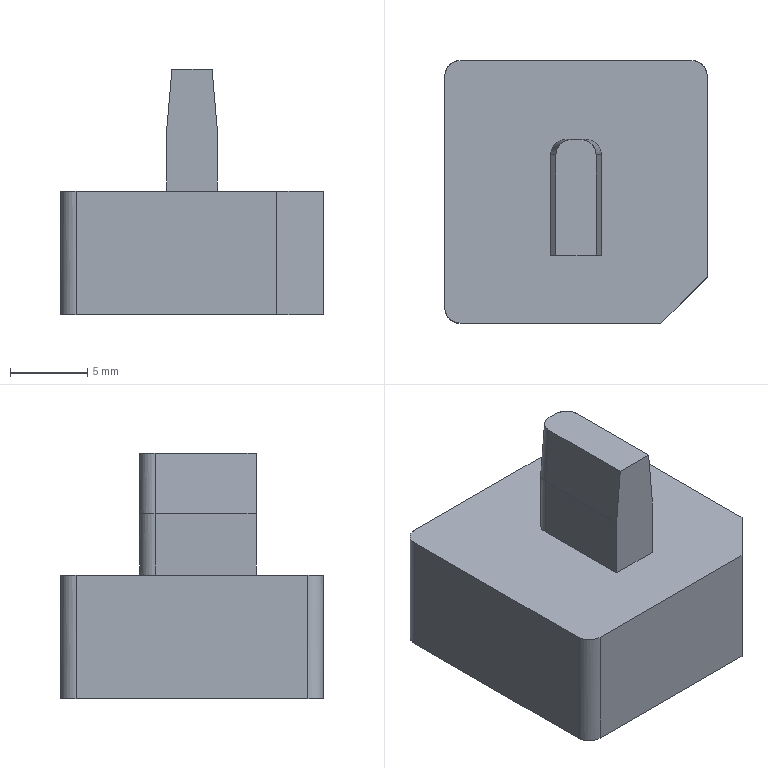NC program | PowerMill | posted with a generic post | part box 17 x 17 x 15.883 mm
Lines 1 to 1090 of 22972:
%
O0001
N104 ( POWERMILL CB  : 2026004.0)
N105 ( POST VER      : 2026.0.0.5161)
N106 ( OPTION FILE   : FANUC)
N107 ( OUTPUT WORKPLANE : WORLD)
N108 (  )
N109 ( TOOL LIST )
N110 (---------------------------------------)
N111 ( NO. | ID        | DIA.| TIP RAD|LENGTH)
N112 (---------------------------------------)
N113 (    1|D10C_1_1   |10.0 |  0.0   |71.32 )
N114 (    3|D10_1_1    |10.0 |  0.0   |71.04 )
N115 (   14|D4_2_1     | 4.0 |  0.0   |62.92 )
N116 (   13|TEXT_D4_1_1| 4.0 |  0.3   |63.16 )
N117 (---------------------------------------)
N118 (  )
N119 ( NUMBER OF TOOLPATHS: 9.0 )
N120 ( ESTIMATED PROGRAM DURATION: 0 HOURS 3 MIN 48 SEC)
N121 (  )
N122 G00 G21 G80 G40 G17
N123 G90
N124 G54
N125 G53 Z0.0
N126 (---------------)
N127 ( START TOOLPATH : 粗公开粗01-扫面平行-D10C )
N128 (---------------)
N129 ( TOOL NO.    :1 )
N130 ( TOOL TYPE   : ENDMILL)
N131 ( TOOL ID     : D10C_1_1)
N132 ( TOOL DIA    : 10.0 LENGTH 71.32)
N133 T1
N134 M6
N135 S8000 M03
N136 G00 G90 X0.0 Y0.0
N137 G43 Z10.2 H1
N138
N139 G05 P10000 R4
N140 X16.15 Y11.15
N141 Z1.004
N142 G01 Z-0.196 F6000.0
N143 X11.15 F10000.0
N144 X-11.15
N145 Y5.575
N146 X11.15
N147 Y0.0
N148 X-11.15
N149 Y-5.575
N150 X11.15
N151 Y-11.15
N152 X-11.15
N153 X-16.15
N154 G00 Z10.2
N155 G05 P0
N156 (---------------)
N157 ( END TOOLPATH : 粗公开粗01-扫面平行-D10C )
N158 (---------------)
N159 ( START TOOLPATH : 粗公开粗01-外形偏置-D10C )
N160 (---------------)
N161 G00 X0.0 Y-0.3245 Z9.8056
N162 G05 P10000 R4
N163 X6.658 Y-17.074
N164 Z0.5698
N165 G01 Z-0.6302 F6000.0
N166 Y-16.5465 F10000.0
N167 G03 X1.9105 Y-11.799 I-4.7475 J0.0
N168 G01 X-10.15
N169 G02 X-11.15 Y-10.799 I0.0 J1.0
N170 G01 Y10.15
N171 G02 X-10.15 Y11.15 I1.0 J0.0
N172 G01 X10.15
N173 G02 X11.15 Y10.15 I0.0 J-1.0
N174 G01 Y-10.799
N175 G02 X10.15 Y-11.799 I-1.0 J0.0
N176 G01 X1.9105
N177 X1.6338 Y-9.2859
N178 X1.5469 Y-9.2955
N179 X-1.5469
N180 X-2.2422 Y-9.2189
N181 X-3.0937 Y-8.9889
N182 X-3.8671 Y-8.6322
N183 X-4.1729 Y-8.4455
N184 X-4.6406 Y-8.0965
N185 X-5.0892 Y-7.6721
N186 X-5.414 Y-7.2898
N187 X-5.6871 Y-6.8986
N188 X-6.088 Y-6.1252
N189 X-6.3397 Y-5.3518
N190 X-6.464 Y-4.5783
N191 X-6.4819 Y-3.8049
N192 Y2.3825
N193 X-6.4242 Y3.1559
N194 X-6.2829 Y3.9293
N195 X-6.1874 Y4.2665
N196 X-6.0257 Y4.7028
N197 X-5.6419 Y5.4762
N198 X-5.414 Y5.8476
N199 X-5.1149 Y6.2496
N200 X-4.3644 Y7.0231
N201 X-3.8671 Y7.4176
N202 X-3.2331 Y7.7965
N203 X-2.3203 Y8.2057
N204 X-1.5469 Y8.4056
N205 X-0.7734 Y8.5178
N206 X0.0 Y8.5371
N207 X0.7734 Y8.5178
N208 X1.5469 Y8.4148
N209 X2.3203 Y8.1997
N210 X3.0937 Y7.8801
N211 X3.8671 Y7.4155
N212 X4.37 Y7.0231
N213 X4.6406 Y6.766
N214 X5.1168 Y6.2496
N215 X5.414 Y5.8419
N216 X5.6452 Y5.4762
N217 X6.0263 Y4.7028
N218 X6.2847 Y3.9293
N219 X6.4278 Y3.1559
N220 X6.4819 Y2.3825
N221 Y-3.8049
N222 X6.464 Y-4.5783
N223 X6.3397 Y-5.3518
N224 X6.088 Y-6.1252
N225 X5.6871 Y-6.8986
N226 X5.414 Y-7.2898
N227 X5.0892 Y-7.6721
N228 X4.6406 Y-8.0965
N229 X4.1729 Y-8.4455
N230 X3.8671 Y-8.6322
N231 X3.0937 Y-8.9889
N232 X2.2422 Y-9.2189
N233 X1.6338 Y-9.2859
N234 X1.9105 Y-11.799
N235 G00 Z3.2356
N236 G01 X6.658 Y-17.074
N237 G00 Z0.1856
N238 G01 Z-1.0144 F6000.0
N239 Y-16.5465 F10000.0
N240 G03 X1.9105 Y-11.799 I-4.7475 J0.0
N241 G01 X1.9062
N242 X1.638 Y-9.287
N243 X1.5469 Y-9.2968
N244 X-1.5469
N245 X-2.2758 Y-9.2189
N246 X-3.0937 Y-9.0008
N247 X-3.8671 Y-8.6507
N248 X-4.2065 Y-8.4455
N249 X-4.6406 Y-8.1239
N250 X-5.1228 Y-7.6721
N251 X-5.414 Y-7.3322
N252 X-5.7207 Y-6.8986
N253 X-6.1217 Y-6.1252
N254 X-6.3733 Y-5.3518
N255 X-6.4976 Y-4.5783
N256 X-6.5155 Y-3.8049
N257 Y2.3825
N258 X-6.4578 Y3.1559
N259 X-6.3166 Y3.9293
N260 X-6.1874 Y4.3673
N261 X-6.0593 Y4.7028
N262 X-5.6755 Y5.4762
N263 X-5.414 Y5.8972
N264 X-5.1485 Y6.2496
N265 X-4.398 Y7.0231
N266 X-3.8671 Y7.4404
N267 X-3.2667 Y7.7965
N268 X-2.3203 Y8.2166
N269 X-1.5469 Y8.4132
N270 X-0.7734 Y8.5205
N271 X0.0 Y8.5371
N272 X0.7734 Y8.5205
N273 X1.5469 Y8.4214
N274 X2.3203 Y8.2118
N275 X3.0937 Y7.8966
N276 X3.8671 Y7.4383
N277 X4.4038 Y7.0231
N278 X4.6406 Y6.7994
N279 X5.1504 Y6.2496
N280 X5.414 Y5.8924
N281 X5.6788 Y5.4762
N282 X6.06 Y4.7028
N283 X6.3183 Y3.9293
N284 X6.4615 Y3.1559
N285 X6.5155 Y2.3825
N286 Y-3.8049
N287 X6.4976 Y-4.5783
N288 X6.3733 Y-5.3518
N289 X6.1217 Y-6.1252
N290 X5.7207 Y-6.8986
N291 X5.414 Y-7.3322
N292 X5.1228 Y-7.6721
N293 X4.6406 Y-8.1239
N294 X4.2065 Y-8.4455
N295 X3.8671 Y-8.6507
N296 X3.0937 Y-9.0008
N297 X2.2758 Y-9.2189
N298 X1.638 Y-9.287
N299 X1.9062 Y-11.799
N300 X-10.15
N301 G02 X-11.15 Y-10.799 I0.0 J1.0
N302 G01 Y10.15
N303 G02 X-10.15 Y11.15 I1.0 J0.0
N304 G01 X10.15
N305 G02 X11.15 Y10.15 I0.0 J-1.0
N306 G01 Y-10.799
N307 G02 X10.15 Y-11.799 I-1.0 J0.0
N308 G01 X1.9105
N309 G00 Z2.8514
N310 G01 X6.658 Y-17.074
N311 G00 Z-0.1986
N312 G01 Z-1.3986 F6000.0
N313 Y-16.5465 F10000.0
N314 G03 X1.9105 Y-11.799 I-4.7475 J0.0
N315 G01 X1.5469
N316 Y-9.2978
N317 X-1.5469
N318 X-2.3094 Y-9.2189
N319 X-3.0937 Y-9.0126
N320 X-3.8671 Y-8.6691
N321 X-4.2401 Y-8.4455
N322 X-4.6406 Y-8.1509
N323 X-5.1564 Y-7.6721
N324 X-5.414 Y-7.3745
N325 X-5.7543 Y-6.8986
N326 X-6.1553 Y-6.1252
N327 X-6.4069 Y-5.3518
N328 X-6.5313 Y-4.5783
N329 X-6.5491 Y-3.8049
N330 Y2.3825
N331 X-6.4914 Y3.1559
N332 X-6.3502 Y3.9293
N333 X-6.0929 Y4.7028
N334 X-5.7092 Y5.4762
N335 X-5.414 Y5.9453
N336 X-5.1821 Y6.2496
N337 X-4.4316 Y7.0231
N338 X-3.8671 Y7.4632
N339 X-3.3003 Y7.7965
N340 X-2.3203 Y8.2276
N341 X-1.5469 Y8.4188
N342 X-0.7734 Y8.5232
N343 X-0.6454
N344 X0.0 Y8.537
N345 X0.6454 Y8.5232
N346 X0.7734
N347 X1.5469 Y8.4278
N348 X2.3203 Y8.2239
N349 X3.0937 Y7.9131
N350 X3.8671 Y7.4611
N351 X4.4376 Y7.0231
N352 X5.184 Y6.2496
N353 X5.414 Y5.9417
N354 X5.7123 Y5.4762
N355 X6.0936 Y4.7028
N356 X6.3519 Y3.9293
N357 X6.4952 Y3.1559
N358 X6.5491 Y2.3825
N359 Y-3.8049
N360 X6.5313 Y-4.5783
N361 X6.4069 Y-5.3518
N362 X6.1874 Y-6.045
N363 X5.7543 Y-6.8986
N364 X5.414 Y-7.3745
N365 X5.1564 Y-7.6721
N366 X4.6406 Y-8.1509
N367 X4.2401 Y-8.4455
N368 X3.8671 Y-8.6691
N369 X3.0937 Y-9.0126
N370 X2.3094 Y-9.2189
N371 X1.5469 Y-9.2978
N372 Y-11.799
N373 X-10.15
N374 G02 X-11.15 Y-10.799 I0.0 J1.0
N375 G01 Y10.15
N376 G02 X-10.15 Y11.15 I1.0 J0.0
N377 G01 X10.15
N378 G02 X11.15 Y10.15 I0.0 J-1.0
N379 G01 Y-10.799
N380 G02 X10.15 Y-11.799 I-1.0 J0.0
N381 G01 X1.9105
N382 G00 Z2.4672
N383 G01 X6.658 Y-17.074
N384 G00 Z-0.5828
N385 G01 Z-1.7828 F6000.0
N386 Y-16.5465 F10000.0
N387 G03 X1.9105 Y-11.799 I-4.7475 J0.0
N388 G01 X1.5469
N389 Y-9.2987
N390 X-1.5469
N391 X-2.3203 Y-9.2229
N392 X-3.0937 Y-9.0244
N393 X-3.8671 Y-8.6876
N394 X-4.2737 Y-8.4455
N395 X-4.6406 Y-8.1779
N396 X-5.1901 Y-7.6721
N397 X-5.414 Y-7.4167
N398 X-5.7879 Y-6.8986
N399 X-6.1874 Y-6.1286
N400 X-6.4405 Y-5.3518
N401 X-6.5649 Y-4.5783
N402 X-6.5827 Y-3.8049
N403 Y2.3825
N404 X-6.525 Y3.1559
N405 X-6.3838 Y3.9293
N406 X-6.1874 Y4.5514
N407 X-5.7428 Y5.4762
N408 X-5.414 Y5.9919
N409 X-5.2157 Y6.2496
N410 X-4.4652 Y7.0231
N411 X-3.8671 Y7.4861
N412 X-3.334 Y7.7965
N413 X-2.3203 Y8.2386
N414 X-1.5469 Y8.4244
N415 X-0.7734 Y8.5255
N416 X-0.5367
N417 X0.0 Y8.537
N418 X0.5367 Y8.5255
N419 X0.7734
N420 X1.5469 Y8.434
N421 X2.3203 Y8.2359
N422 X3.0937 Y7.9295
N423 X3.3547 Y7.7965
N424 X3.8671 Y7.4839
N425 X4.4714 Y7.0231
N426 X5.2176 Y6.2496
N427 X5.414 Y5.9891
N428 X5.7459 Y5.4762
N429 X6.1273 Y4.7028
N430 X6.3854 Y3.9293
N431 X6.529 Y3.1559
N432 X6.5827 Y2.3825
N433 Y-3.8049
N434 X6.5649 Y-4.5783
N435 X6.4405 Y-5.3518
N436 X6.1889 Y-6.1252
N437 X5.7879 Y-6.8986
N438 X5.414 Y-7.4167
N439 X5.1901 Y-7.6721
N440 X4.6406 Y-8.1779
N441 X4.2737 Y-8.4455
N442 X3.8671 Y-8.6876
N443 X3.0937 Y-9.0244
N444 X2.3431 Y-9.2189
N445 X1.5469 Y-9.2987
N446 Y-11.799
N447 X-10.15
N448 G02 X-11.15 Y-10.799 I0.0 J1.0
N449 G01 Y10.15
N450 G02 X-10.15 Y11.15 I1.0 J0.0
N451 G01 X10.15
N452 G02 X11.15 Y10.15 I0.0 J-1.0
N453 G01 Y-10.799
N454 G02 X10.15 Y-11.799 I-1.0 J0.0
N455 G01 X1.9105
N456 G00 Z2.083
N457 G01 X6.658 Y-17.074
N458 G00 Z-0.967
N459 G01 Z-2.167 F6000.0
N460 Y-16.5465 F10000.0
N461 G03 X1.9105 Y-11.799 I-4.7475 J0.0
N462 G01 X1.5469
N463 Y-9.2993
N464 X-1.5469
N465 X-2.3203 Y-9.2287
N466 X-3.0937 Y-9.0359
N467 X-3.8671 Y-8.7061
N468 X-4.3073 Y-8.4455
N469 X-4.6406 Y-8.2049
N470 X-5.2237 Y-7.6721
N471 X-5.414 Y-7.4566
N472 X-5.8215 Y-6.8986
N473 X-6.1874 Y-6.2076
N474 X-6.4741 Y-5.3518
N475 X-6.5985 Y-4.5783
N476 X-6.6163 Y-3.8049
N477 Y2.3825
N478 X-6.5586 Y3.1559
N479 X-6.4175 Y3.9293
N480 X-6.1874 Y4.6368
N481 X-5.7764 Y5.4762
N482 X-5.414 Y6.0386
N483 X-5.2493 Y6.2496
N484 X-4.4988 Y7.0231
N485 X-3.8671 Y7.5089
N486 X-3.0937 Y7.9343
N487 X-2.3203 Y8.2495
N488 X-1.5469 Y8.4297
N489 X-0.7734 Y8.5277
N490 X-0.4309
N491 X0.0 Y8.5369
N492 X0.4309 Y8.5277
N493 X0.7734
N494 X1.5469 Y8.4401
N495 X2.3203 Y8.2479
N496 X3.0937 Y7.946
N497 X3.3886 Y7.7965
N498 X3.8671 Y7.5067
N499 X4.5052 Y7.0231
N500 X5.2512 Y6.2496
N501 X5.7794 Y5.4762
N502 X6.161 Y4.7028
N503 X6.419 Y3.9293
N504 X6.5627 Y3.1559
N505 X6.6163 Y2.3825
N506 Y-3.8049
N507 X6.5985 Y-4.5783
N508 X6.4741 Y-5.3518
N509 X6.2225 Y-6.1252
N510 X5.8215 Y-6.8986
N511 X5.414 Y-7.4566
N512 X5.2237 Y-7.6721
N513 X4.6406 Y-8.2049
N514 X4.3073 Y-8.4455
N515 X3.8671 Y-8.7061
N516 X3.0937 Y-9.0359
N517 X2.3767 Y-9.2189
N518 X1.5469 Y-9.2993
N519 Y-11.799
N520 X-10.15
N521 G02 X-11.15 Y-10.799 I0.0 J1.0
N522 G01 Y10.15
N523 G02 X-10.15 Y11.15 I1.0 J0.0
N524 G01 X10.15
N525 G02 X11.15 Y10.15 I0.0 J-1.0
N526 G01 Y-10.799
N527 G02 X10.15 Y-11.799 I-1.0 J0.0
N528 G01 X1.9105
N529 G00 Z1.6988
N530 G01 X6.658 Y-17.074
N531 G00 Z-1.3512
N532 G01 Z-2.5512 F6000.0
N533 Y-16.5465 F10000.0
N534 G03 X1.9105 Y-11.799 I-4.7475 J0.0
N535 G01 X1.5469
N536 Y-9.2998
N537 X-1.5469
N538 X-2.3203 Y-9.2342
N539 X-3.0937 Y-9.0465
N540 X-3.8671 Y-8.7232
N541 X-4.341 Y-8.4455
N542 X-4.6406 Y-8.2312
N543 X-5.2573 Y-7.6721
N544 X-5.414 Y-7.4962
N545 X-5.8551 Y-6.8986
N546 X-6.1874 Y-6.2822
N547 X-6.5078 Y-5.3518
N548 X-6.6321 Y-4.5783
N549 X-6.6499 Y-3.8049
N550 Y2.3825
N551 X-6.5922 Y3.1559
N552 X-6.4511 Y3.9293
N553 X-6.1938 Y4.7028
N554 X-5.81 Y5.4762
N555 X-5.283 Y6.2496
N556 X-4.6406 Y6.9227
N557 X-3.8671 Y7.53
N558 X-3.0937 Y7.9511
N559 X-2.3203 Y8.2605
N560 X-1.5469 Y8.435
N561 X-0.7734 Y8.5295
N562 X-0.3421
N563 X0.0 Y8.5369
N564 X0.3421 Y8.5295
N565 X0.7734
N566 X1.5469 Y8.446
N567 X2.3203 Y8.2582
N568 X3.0937 Y7.9616
N569 X3.4224 Y7.7965
N570 X3.8671 Y7.5295
N571 X4.539 Y7.0231
N572 X5.2848 Y6.2496
N573 X5.813 Y5.4762
N574 X6.1874 Y4.7204
N575 X6.4526 Y3.9293
N576 X6.5964 Y3.1559
N577 X6.6499 Y2.3825
N578 Y-3.8049
N579 X6.6321 Y-4.5783
N580 X6.5078 Y-5.3518
N581 X6.2561 Y-6.1252
N582 X5.8551 Y-6.8986
N583 X5.414 Y-7.4962
N584 X5.2573 Y-7.6721
N585 X4.6406 Y-8.2312
N586 X4.341 Y-8.4455
N587 X3.8671 Y-8.7232
N588 X3.0937 Y-9.0465
N589 X2.4103 Y-9.2189
N590 X1.5469 Y-9.2998
N591 Y-11.799
N592 X-10.15
N593 G02 X-11.15 Y-10.799 I0.0 J1.0
N594 G01 Y10.15
N595 G02 X-10.15 Y11.15 I1.0 J0.0
N596 G01 X10.15
N597 G02 X11.15 Y10.15 I0.0 J-1.0
N598 G01 Y-10.799
N599 G02 X10.15 Y-11.799 I-1.0 J0.0
N600 G01 X1.9105
N601 G00 Z1.3146
N602 G01 X6.658 Y-17.074
N603 G00 Z-1.7354
N604 G01 Z-2.9354 F6000.0
N605 Y-16.5465 F10000.0
N606 G03 X1.9105 Y-11.799 I-4.7475 J0.0
N607 G01 X1.5469
N608 Y-9.3
N609 X-1.5469
N610 X-2.3203 Y-9.2395
N611 X-3.0937 Y-9.0571
N612 X-3.8671 Y-8.74
N613 X-4.3746 Y-8.4455
N614 X-4.6406 Y-8.2563
N615 X-5.2909 Y-7.6721
N616 X-5.8887 Y-6.8986
N617 X-6.2897 Y-6.1252
N618 X-6.5414 Y-5.3518
N619 X-6.6657 Y-4.5783
N620 X-6.6836 Y-3.8049
N621 Y2.3825
N622 X-6.6258 Y3.1559
N623 X-6.4847 Y3.9293
N624 X-6.2277 Y4.7028
N625 X-5.8436 Y5.4762
N626 X-5.414 Y6.1267
N627 X-4.6406 Y6.9541
N628 X-3.8671 Y7.551
N629 X-3.0937 Y7.9679
N630 X-2.3203 Y8.2705
N631 X-1.5469 Y8.4403
N632 X-0.7734 Y8.5313
N633 X-0.2572
N634 X0.0 Y8.5368
N635 X0.2572 Y8.5313
N636 X0.7734
N637 X1.5469 Y8.4516
N638 X2.3203 Y8.2684
N639 X3.0937 Y7.9768
N640 X3.4562 Y7.7965
N641 X3.8671 Y7.5516
N642 X4.5728 Y7.0231
N643 X5.3184 Y6.2496
N644 X5.8466 Y5.4762
N645 X6.1874 Y4.8031
N646 X6.4862 Y3.9293
N647 X6.6301 Y3.1559
N648 X6.6836 Y2.3825
N649 Y-3.8049
N650 X6.6657 Y-4.5783
N651 X6.5414 Y-5.3518
N652 X6.2897 Y-6.1252
N653 X5.8887 Y-6.8986
N654 X5.2909 Y-7.6721
N655 X4.6406 Y-8.2563
N656 X4.3746 Y-8.4455
N657 X3.8671 Y-8.74
N658 X3.0937 Y-9.0571
N659 X2.4439 Y-9.2189
N660 X1.5469 Y-9.3
N661 Y-11.799
N662 X-10.15
N663 G02 X-11.15 Y-10.799 I0.0 J1.0
N664 G01 Y10.15
N665 G02 X-10.15 Y11.15 I1.0 J0.0
N666 G01 X10.15
N667 G02 X11.15 Y10.15 I0.0 J-1.0
N668 G01 Y-10.799
N669 G02 X10.15 Y-11.799 I-1.0 J0.0
N670 G01 X1.9105
N671 G00 Z0.9304
N672 G01 X6.658 Y-17.074
N673 G00 Z-2.1196
N674 G01 Z-3.3196 F6000.0
N675 Y-16.5465 F10000.0
N676 G03 X1.9105 Y-11.799 I-4.7475 J0.0
N677 G01 X1.5469
N678 Y-9.3
N679 X-1.5469
N680 X-2.3203 Y-9.2445
N681 X-3.0937 Y-9.0677
N682 X-3.8671 Y-8.7569
N683 X-4.4082 Y-8.4455
N684 X-4.6406 Y-8.2813
N685 X-5.3245 Y-7.6721
N686 X-5.9223 Y-6.8986
N687 X-6.1874 Y-6.4245
N688 X-6.3233 Y-6.1252
N689 X-6.575 Y-5.3518
N690 X-6.6993 Y-4.5783
N691 X-6.7172 Y-3.8049
N692 Y2.3825
N693 X-6.6595 Y3.1559
N694 X-6.5184 Y3.9293
N695 X-6.2616 Y4.7028
N696 X-5.8772 Y5.4762
N697 X-5.414 Y6.1704
N698 X-4.6406 Y6.9852
N699 X-3.8671 Y7.572
N700 X-3.0937 Y7.9846
N701 X-2.3203 Y8.2803
N702 X-1.5469 Y8.4456
N703 X-0.7734 Y8.5328
N704 X-0.1853
N705 X0.0 Y8.5368
N706 X0.1853 Y8.5328
N707 X0.7734
N708 X1.5469 Y8.4572
N709 X2.3203 Y8.2787
N710 X3.0937 Y7.9921
N711 X3.4901 Y7.7965
N712 X3.8671 Y7.5733
N713 X4.6066 Y7.0231
N714 X5.352 Y6.2496
N715 X5.8801 Y5.4762
N716 X6.1874 Y4.8812
N717 X6.5197 Y3.9293
N718 X6.6638 Y3.1559
N719 X6.7172 Y2.3825
N720 Y-3.8049
N721 X6.6993 Y-4.5783
N722 X6.575 Y-5.3518
N723 X6.3233 Y-6.1252
N724 X6.1874 Y-6.4245
N725 X5.9223 Y-6.8986
N726 X5.414 Y-7.5734
N727 X4.6406 Y-8.2813
N728 X4.4082 Y-8.4455
N729 X3.8671 Y-8.7569
N730 X3.0937 Y-9.0677
N731 X2.4775 Y-9.2189
N732 X1.5469 Y-9.3
N733 Y-11.799
N734 X-10.15
N735 G02 X-11.15 Y-10.799 I0.0 J1.0
N736 G01 Y10.15
N737 G02 X-10.15 Y11.15 I1.0 J0.0
N738 G01 X10.15
N739 G02 X11.15 Y10.15 I0.0 J-1.0
N740 G01 Y-10.799
N741 G02 X10.15 Y-11.799 I-1.0 J0.0
N742 G01 X1.9105
N743 G00 Z0.5462
N744 G01 X6.658 Y-17.074
N745 G00 Z-2.5038
N746 G01 Z-3.7038 F6000.0
N747 Y-16.5465 F10000.0
N748 G03 X1.9105 Y-11.799 I-4.7475 J0.0
N749 G01 X1.5469
N750 Y-9.3
N751 X-1.5469
N752 X-2.3203 Y-9.2495
N753 X-3.0937 Y-9.0782
N754 X-3.8671 Y-8.7738
N755 X-4.4418 Y-8.4455
N756 X-4.6406 Y-8.3064
N757 X-5.3581 Y-7.6721
N758 X-5.956 Y-6.8986
N759 X-6.1874 Y-6.4912
N760 X-6.3569 Y-6.1252
N761 X-6.6086 Y-5.3518
N762 X-6.7329 Y-4.5783
N763 X-6.7508 Y-3.8049
N764 Y2.3825
N765 X-6.6931 Y3.1559
N766 X-6.552 Y3.9293
N767 X-6.2955 Y4.7028
N768 X-5.9108 Y5.4762
N769 X-5.414 Y6.2122
N770 X-4.6406 Y7.0163
N771 X-3.8671 Y7.593
N772 X-3.0937 Y8.0009
N773 X-2.3203 Y8.2901
N774 X-1.5469 Y8.4509
N775 X-0.7734 Y8.534
N776 X-0.1248
N777 X0.0 Y8.5367
N778 X0.1248 Y8.534
N779 X0.7734
N780 X1.5469 Y8.4624
N781 X2.3203 Y8.2889
N782 X3.0937 Y8.0073
N783 X3.5239 Y7.7965
N784 X3.8671 Y7.5949
N785 X4.6404 Y7.0231
N786 X5.3857 Y6.2496
N787 X5.9137 Y5.4762
N788 X6.1874 Y4.957
N789 X6.2957 Y4.7028
N790 X6.5533 Y3.9293
N791 X6.6975 Y3.1559
N792 X6.7508 Y2.3825
N793 Y-3.8049
N794 X6.7329 Y-4.5783
N795 X6.6086 Y-5.3518
N796 X6.3569 Y-6.1252
N797 X6.1874 Y-6.4912
N798 X5.956 Y-6.8986
N799 X5.414 Y-7.6107
N800 X4.6406 Y-8.3064
N801 X4.4418 Y-8.4455
N802 X3.8671 Y-8.7738
N803 X3.0937 Y-9.0782
N804 X2.5111 Y-9.2189
N805 X1.5469 Y-9.3
N806 Y-11.799
N807 X-10.15
N808 G02 X-11.15 Y-10.799 I0.0 J1.0
N809 G01 Y10.15
N810 G02 X-10.15 Y11.15 I1.0 J0.0
N811 G01 X10.15
N812 G02 X11.15 Y10.15 I0.0 J-1.0
N813 G01 Y-10.799
N814 G02 X10.15 Y-11.799 I-1.0 J0.0
N815 G01 X1.9105
N816 G00 Z0.162
N817 G01 X6.658 Y-17.074
N818 G00 Z-2.888
N819 G01 Z-4.088 F6000.0
N820 Y-16.5465 F10000.0
N821 G03 X1.9105 Y-11.799 I-4.7475 J0.0
N822 G01 X-10.15
N823 G02 X-11.15 Y-10.799 I0.0 J1.0
N824 G01 Y10.15
N825 G02 X-10.15 Y11.15 I1.0 J0.0
N826 G01 X10.15
N827 G02 X11.15 Y10.15 I0.0 J-1.0
N828 G01 Y-10.799
N829 G02 X10.15 Y-11.799 I-1.0 J0.0
N830 G01 X1.9861
N831 X1.8369 Y-9.2828
N832 X1.5469 Y-9.3
N833 X-1.5469
N834 X-2.3203 Y-9.2541
N835 X-3.0937 Y-9.0888
N836 X-3.8671 Y-8.7907
N837 X-4.6406 Y-8.3314
N838 X-5.3917 Y-7.6721
N839 X-5.9896 Y-6.8986
N840 X-6.1874 Y-6.5565
N841 X-6.3906 Y-6.1252
N842 X-6.6422 Y-5.3518
N843 X-6.7666 Y-4.5783
N844 X-6.7844 Y-3.8049
N845 Y2.3825
N846 X-6.7267 Y3.1559
N847 X-6.5857 Y3.9293
N848 X-6.3294 Y4.7028
N849 X-5.9444 Y5.4762
N850 X-5.4174 Y6.2496
N851 X-4.6406 Y7.0474
N852 X-3.8671 Y7.614
N853 X-3.0937 Y8.0166
N854 X-2.3203 Y8.2999
N855 X-1.5469 Y8.4562
N856 X-0.7734 Y8.5351
N857 X-0.0707
N858 X0.0 Y8.5367
N859 X0.0704 Y8.5351
N860 X0.7734 Y8.5352
N861 X1.5469 Y8.4676
N862 X2.3203 Y8.3
N863 X3.0937 Y8.0226
N864 X3.5577 Y7.7965
N865 X3.8671 Y7.6166
N866 X4.6406 Y7.052
N867 X5.414 Y6.2562
N868 X5.9472 Y5.4762
N869 X6.1874 Y5.0293
N870 X6.3294 Y4.7028
N871 X6.587 Y3.9293
N872 X6.7312 Y3.1559
N873 X6.7844 Y2.3825
N874 Y-3.8049
N875 X6.7666 Y-4.5783
N876 X6.6422 Y-5.3518
N877 X6.3906 Y-6.1252
N878 X6.1874 Y-6.5565
N879 X5.9896 Y-6.8986
N880 X5.414 Y-7.648
N881 X4.6406 Y-8.3314
N882 X3.8671 Y-8.7907
N883 X3.0937 Y-9.0888
N884 X2.5447 Y-9.2189
N885 X2.3203 Y-9.2541
N886 X1.8369 Y-9.2828
N887 X1.9861 Y-11.799
N888 X1.9105
N889 G00 Z-0.2222
N890 G01 X6.658 Y-17.074
N891 G00 Z-3.2722
N892 G01 Z-4.4722 F6000.0
N893 Y-16.5465 F10000.0
N894 G03 X1.9105 Y-11.799 I-4.7475 J0.0
N895 G01 X-10.15
N896 G02 X-11.15 Y-10.799 I0.0 J1.0
N897 G01 Y10.15
N898 G02 X-10.15 Y11.15 I1.0 J0.0
N899 G01 X10.15
N900 G02 X11.15 Y10.15 I0.0 J-1.0
N901 G01 Y-10.799
N902 G02 X10.15 Y-11.799 I-1.0 J0.0
N903 G01 X1.984
N904 X1.8369 Y-9.283
N905 X1.5469 Y-9.3
N906 X-1.5469
N907 X-2.3203 Y-9.2547
N908 X-3.0937 Y-9.0903
N909 X-3.8671 Y-8.7931
N910 X-4.6406 Y-8.3349
N911 X-5.3964 Y-7.6721
N912 X-5.9942 Y-6.8986
N913 X-6.1874 Y-6.5655
N914 X-6.3952 Y-6.1252
N915 X-6.6469 Y-5.3518
N916 X-6.7712 Y-4.5783
N917 X-6.7891 Y-3.8049
N918 Y2.3825
N919 X-6.7379 Y3.1559
N920 X-6.5904 Y3.9293
N921 X-6.3361 Y4.7028
N922 X-5.9524 Y5.4762
N923 X-5.4219 Y6.2496
N924 X-4.6747 Y7.0231
N925 X-3.8671 Y7.6198
N926 X-3.0937 Y8.0247
N927 X-2.3203 Y8.3012
N928 X-1.5469 Y8.4678
N929 X-0.7734 Y8.5352
N930 X-0.0583 Y8.5354
N931 X0.0 Y8.5366
N932 X0.0574 Y8.5354
N933 X0.7734 Y8.5355
N934 X1.5469 Y8.469
N935 X2.3203 Y8.302
N936 X3.0937 Y8.0247
N937 X3.1554 Y7.9924
N938 X3.5577 Y7.7964
N939 X3.8 Y7.6556
N940 X3.8671 Y7.6205
N941 X4.6406 Y7.056
N942 X5.414 Y6.2619
N943 X5.955 Y5.4762
N944 X6.1874 Y5.0392
N945 X6.3361 Y4.7028
N946 X6.5918 Y3.9293
N947 X6.7397 Y3.1559
N948 X6.7891 Y2.3825
N949 Y-3.8049
N950 X6.7712 Y-4.5783
N951 X6.6469 Y-5.3518
N952 X6.3952 Y-6.1252
N953 X6.1874 Y-6.5655
N954 X5.9942 Y-6.8986
N955 X5.414 Y-7.6531
N956 X4.6406 Y-8.3349
N957 X3.8671 Y-8.7931
N958 X3.0937 Y-9.0903
N959 X2.5494 Y-9.2189
N960 X2.3203 Y-9.2547
N961 X1.8369 Y-9.283
N962 X1.984 Y-11.799
N963 X1.9105
N964 G00 Z-0.6064
N965 G01 X6.658 Y-17.074
N966 G00 Z-3.6564
N967 G01 Z-4.8564 F6000.0
N968 Y-16.5465 F10000.0
N969 G03 X1.9105 Y-11.799 I-4.7475 J0.0
N970 G01 X-10.15
N971 G02 X-11.15 Y-10.799 I0.0 J1.0
N972 G01 Y10.15
N973 G02 X-10.15 Y11.15 I1.0 J0.0
N974 G01 X10.15
N975 G02 X11.15 Y10.15 I0.0 J-1.0
N976 G01 Y-10.799
N977 G02 X10.15 Y-11.799 I-1.0 J0.0
N978 G01 X1.984
N979 X1.8369 Y-9.283
N980 X1.5469 Y-9.3
N981 X-1.5469
N982 X-2.3203 Y-9.2548
N983 X-3.0937 Y-9.0903
N984 X-3.8671 Y-8.7931
N985 X-4.6406 Y-8.3349
N986 X-5.3964 Y-7.6721
N987 X-5.9942 Y-6.8986
N988 X-6.1874 Y-6.5655
N989 X-6.3952 Y-6.1252
N990 X-6.6469 Y-5.3518
N991 X-6.7712 Y-4.5783
N992 X-6.7891 Y-3.8049
N993 Y2.3825
N994 X-6.7382 Y3.1559
N995 X-6.5905 Y3.9293
N996 X-6.3361 Y4.7028
N997 X-5.9538 Y5.4762
N998 X-5.422 Y6.2496
N999 X-4.6747 Y7.0231
N1000 X-3.8671 Y7.6198
N1001 X-3.0937 Y8.0247
N1002 X-2.3203 Y8.3012
N1003 X-1.5469 Y8.4678
N1004 X-0.7734 Y8.5352
N1005 X-0.0556 Y8.5354
N1006 X0.0 Y8.5366
N1007 X0.0547 Y8.5354
N1008 X0.7734 Y8.5355
N1009 X1.5469 Y8.469
N1010 X2.3203 Y8.302
N1011 X3.0937 Y8.0247
N1012 X3.1572 Y7.9915
N1013 X3.5577 Y7.7964
N1014 X3.7988 Y7.6562
N1015 X3.8671 Y7.6205
N1016 X4.6406 Y7.056
N1017 X5.414 Y6.2619
N1018 X5.955 Y5.4762
N1019 X6.1874 Y5.0392
N1020 X6.3361 Y4.7028
N1021 X6.5918 Y3.9293
N1022 X6.7397 Y3.1559
N1023 X6.7891 Y2.3825
N1024 Y-3.8049
N1025 X6.7712 Y-4.5783
N1026 X6.6469 Y-5.3518
N1027 X6.3952 Y-6.1252
N1028 X6.1874 Y-6.5655
N1029 X5.9942 Y-6.8986
N1030 X5.414 Y-7.6531
N1031 X4.6406 Y-8.3349
N1032 X3.8671 Y-8.7931
N1033 X3.0937 Y-9.0903
N1034 X2.5494 Y-9.2189
N1035 X2.3203 Y-9.2548
N1036 X1.8369 Y-9.283
N1037 X1.984 Y-11.799
N1038 X1.9105
N1039 G00 Z-0.9906
N1040 G01 X6.658 Y-17.074
N1041 G00 Z-4.0406
N1042 G01 Z-5.2406 F6000.0
N1043 Y-16.5465 F10000.0
N1044 G03 X1.9105 Y-11.799 I-4.7475 J0.0
N1045 G01 X-10.15
N1046 G02 X-11.15 Y-10.799 I0.0 J1.0
N1047 G01 Y10.15
N1048 G02 X-10.15 Y11.15 I1.0 J0.0
N1049 G01 X10.15
N1050 G02 X11.15 Y10.15 I0.0 J-1.0
N1051 G01 Y-10.799
N1052 G02 X10.15 Y-11.799 I-1.0 J0.0
N1053 G01 X1.984
N1054 X1.8369 Y-9.283
N1055 X1.5469 Y-9.3
N1056 X-1.5469
N1057 X-2.3203 Y-9.2548
N1058 X-3.0937 Y-9.0903
N1059 X-3.8671 Y-8.7931
N1060 X-4.6406 Y-8.3349
N1061 X-5.3964 Y-7.6721
N1062 X-5.9942 Y-6.8986
N1063 X-6.1874 Y-6.5655
N1064 X-6.3952 Y-6.1252
N1065 X-6.6469 Y-5.3518
N1066 X-6.7712 Y-4.5783
N1067 X-6.7891 Y-3.8049
N1068 Y2.3825
N1069 X-6.7386 Y3.1559
N1070 X-6.5906 Y3.9293
N1071 X-6.3361 Y4.7028
N1072 X-5.954 Y5.4762
N1073 X-5.422 Y6.2496
N1074 X-4.6747 Y7.0231
N1075 X-3.8671 Y7.6198
N1076 X-3.0937 Y8.0247
N1077 X-2.3203 Y8.3012
N1078 X-1.5469 Y8.4678
N1079 X-0.7734 Y8.5353
N1080 X-0.0528 Y8.5354
N1081 X0.0 Y8.5365
N1082 X0.052 Y8.5354
N1083 X0.7734 Y8.5355
N1084 X1.5469 Y8.469
N1085 X2.3203 Y8.302
N1086 X3.0937 Y8.0247
N1087 X3.159 Y7.9906
N1088 X3.5577 Y7.7963
N1089 X3.7977 Y7.6568
N1090 X3.8671 Y7.6205
N1091 X4.6406 Y7.056
N1092 X5.414 Y6.2619
N1093 X5.955 Y5.4762
N1094 X6.1874 Y5.0392
N1095 X6.3361 Y4.7028
N1096 X6.5918 Y3.9293
N1097 X6.7397 Y3.1559
N1098 X6.7891 Y2.3825
N1099 Y-3.8049
N1100 X6.7712 Y-4.5783
N1101 X6.6469 Y-5.3518
N1102 X6.3952 Y-6.1252
N1103 X6.1874 Y-6.5655
N1104 X5.9942 Y-6.8986
N1105 X5.414 Y-7.6531
N1106 X4.6406 Y-8.3349
N1107 X3.8671 Y-8.7931
N1108 X3.0937 Y-9.0903
N1109 X2.5494 Y-9.2189
N1110 X2.3203 Y-9.2548
N1111 X1.8369 Y-9.283
N1112 X1.984 Y-11.799
N1113 X1.9105
N1114 G00 Z-1.3748
N1115 G01 X6.658 Y-17.074
N1116 G00 Z-4.4248
N1117 G01 Z-5.6248 F6000.0
N1118 Y-16.5465 F10000.0
N1119 G03 X1.9105 Y-11.799 I-4.7475 J0.0
N1120 G01 X-10.15
N1121 G02 X-11.15 Y-10.799 I0.0 J1.0
N1122 G01 Y10.15
N1123 G02 X-10.15 Y11.15 I1.0 J0.0
N1124 G01 X10.15
N1125 G02 X11.15 Y10.15 I0.0 J-1.0
N1126 G01 Y-10.799
N1127 G02 X10.15 Y-11.799 I-1.0 J0.0
N1128 G01 X1.984
N1129 X1.8369 Y-9.283
N1130 X1.5469 Y-9.3
N1131 X-1.5469
N1132 X-2.3203 Y-9.2548
N1133 X-3.0937 Y-9.0903
N1134 X-3.8671 Y-8.7931
N1135 X-4.6406 Y-8.3349
N1136 X-5.3964 Y-7.6721
N1137 X-5.9942 Y-6.8986
N1138 X-6.1874 Y-6.5655
N1139 X-6.3952 Y-6.1252
N1140 X-6.6469 Y-5.3518
N1141 X-6.7712 Y-4.5783
N1142 X-6.7891 Y-3.8049
N1143 Y2.3825
N1144 X-6.7389 Y3.1559
N1145 X-6.5907 Y3.9293
N1146 X-6.3361 Y4.7028
N1147 X-5.9541 Y5.4762
N1148 X-5.422 Y6.2496
N1149 X-4.6747 Y7.0231
N1150 X-3.8671 Y7.6198
N1151 X-3.0937 Y8.0247
N1152 X-2.3203 Y8.3012
N1153 X-1.5469 Y8.4678
N1154 X-0.7734 Y8.5353
N1155 X-0.0501 Y8.5354
N1156 X0.0 Y8.5365
N1157 X0.0493 Y8.5354
N1158 X0.7734 Y8.5355
N1159 X1.5469 Y8.469
N1160 X2.3203 Y8.302
N1161 X3.0937 Y8.0247
N1162 X3.1609 Y7.9896
N1163 X3.5576 Y7.7963
N1164 X3.7966 Y7.6574
N1165 X3.8671 Y7.6205
N1166 X4.6406 Y7.056
N1167 X5.414 Y6.2619
N1168 X5.955 Y5.4762
N1169 X6.1874 Y5.0392
N1170 X6.3361 Y4.7028
N1171 X6.5918 Y3.9293
N1172 X6.7397 Y3.1559
N1173 X6.7891 Y2.3825
N1174 Y-3.8049
N1175 X6.7712 Y-4.5783
N1176 X6.6469 Y-5.3518
N1177 X6.3952 Y-6.1252
N1178 X6.1874 Y-6.5655
N1179 X5.9942 Y-6.8986
N1180 X5.414 Y-7.6532
N1181 X4.6406 Y-8.3349
N1182 X3.8671 Y-8.7931
N1183 X3.0937 Y-9.0903
N1184 X2.5494 Y-9.2189
N1185 X2.3203 Y-9.2548
N1186 X1.8369 Y-9.283
N1187 X1.984 Y-11.799